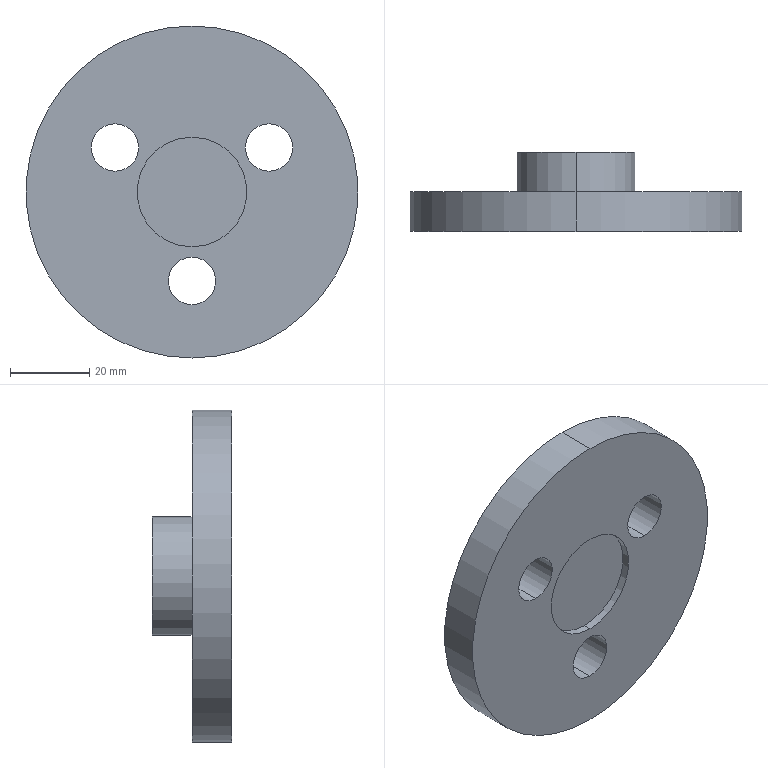Part | SolidWorks | features ICE 3, CirPattern 1, Extrusion 1 | 1 solid | 81 faces | box 84 x 20 x 84 mm | volume 50141 mm3 | cylinder 44 | spline 32 | plane 5 | commonest cylinder face diameters 27.75 x18 23.25 x16 12 x6 30 x2 84 x2